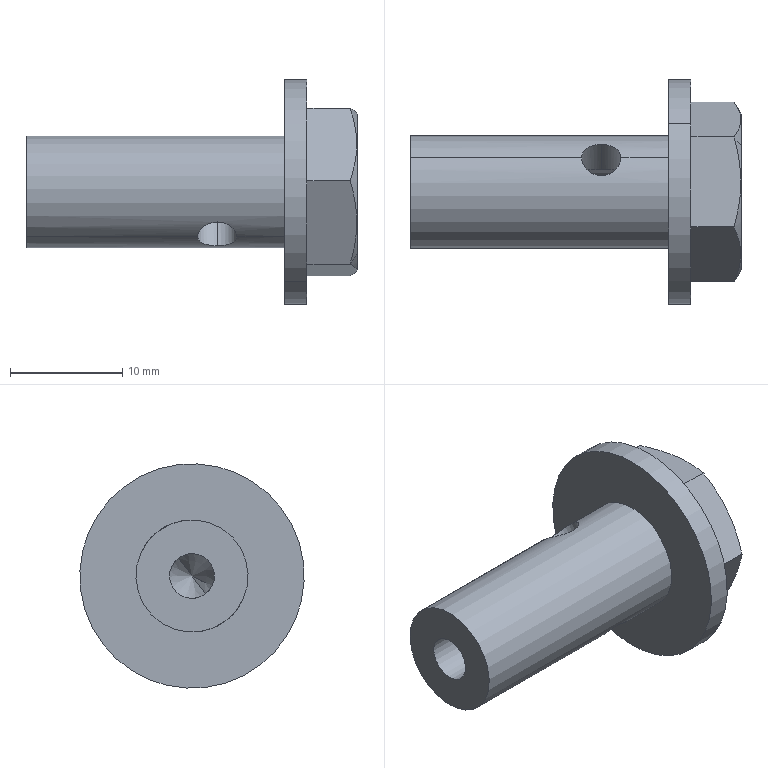Part | SolidWorks | features BaseBody 1 | 1 solid | 24 faces | box 29.5 x 20 x 20 mm | volume 2879 mm3 | cylinder 10 | plane 10 | cone 4 | commonest cylinder face diameters 3.5 x4 4 x2 10 x2 20 x2
STEP:
#1=CARTESIAN_POINT('',(8.537,-14.052,-30.789));
#2=VERTEX_POINT('',#1);
#3=CARTESIAN_POINT('',(8.537,-26.156,-46.711));
#4=VERTEX_POINT('',#3);
#5=CARTESIAN_POINT('',(8.537,-20.104,-38.75));
#6=DIRECTION('',(1.,0.,0.));
#7=DIRECTION('',(0.,0.6052,0.7961));
#8=AXIS2_PLACEMENT_3D('',#5,#6,#7);
#9=CIRCLE('',#8,10.);
#10=EDGE_CURVE('',#2,#4,#9,.T.);
#11=ORIENTED_EDGE('',*,*,#10,.T.);
#12=CARTESIAN_POINT('',(10.537,-26.156,-46.711));
#13=VERTEX_POINT('',#12);
#14=CARTESIAN_POINT('',(15.037,-26.156,-46.711));
#15=DIRECTION('',(1.,0.,0.));
#16=VECTOR('',#15,1000.);
#17=LINE('',#14,#16);
#18=EDGE_CURVE('',#4,#13,#17,.T.);
#19=ORIENTED_EDGE('',*,*,#18,.T.);
#20=CARTESIAN_POINT('',(10.537,-14.052,-30.789));
#21=VERTEX_POINT('',#20);
#22=CARTESIAN_POINT('',(10.537,-20.104,-38.75));
#23=DIRECTION('',(1.,0.,0.));
#24=DIRECTION('',(0.,-0.6052,-0.7961));
#25=AXIS2_PLACEMENT_3D('',#22,#23,#24);
#26=CIRCLE('',#25,10.);
#27=EDGE_CURVE('',#21,#13,#26,.T.);
#28=ORIENTED_EDGE('',*,*,#27,.F.);
#29=CARTESIAN_POINT('',(15.037,-14.052,-30.789));
#30=DIRECTION('',(1.,0.,0.));
#31=VECTOR('',#30,1000.);
#32=LINE('',#29,#31);
#33=EDGE_CURVE('',#2,#21,#32,.T.);
#34=ORIENTED_EDGE('',*,*,#33,.F.);
#35=EDGE_LOOP('',(#11,#19,#28,#34));
#36=FACE_OUTER_BOUND('',#35,.T.);
#37=CARTESIAN_POINT('',(15.037,-20.104,-38.75));
#38=DIRECTION('',(1.,0.,0.));
#39=DIRECTION('',(0.,0.6052,0.7961));
#40=AXIS2_PLACEMENT_3D('',#37,#38,#39);
#41=CYLINDRICAL_SURFACE('',#40,10.);
#42=ADVANCED_FACE('',(#36),#41,.T.);
#43=CARTESIAN_POINT('',(-14.463,-17.078,-34.77));
#44=VERTEX_POINT('',#43);
#45=CARTESIAN_POINT('',(-14.463,-23.13,-42.73));
#46=VERTEX_POINT('',#45);
#47=CARTESIAN_POINT('',(-14.463,-20.104,-38.75));
#48=DIRECTION('',(1.,0.,0.));
#49=DIRECTION('',(0.,0.6052,0.7961));
#50=AXIS2_PLACEMENT_3D('',#47,#48,#49);
#51=CIRCLE('',#50,5.);
#52=EDGE_CURVE('',#44,#46,#51,.T.);
#53=ORIENTED_EDGE('',*,*,#52,.T.);
#54=CARTESIAN_POINT('',(0.7871,-23.13,-42.73));
#55=VERTEX_POINT('',#54);
#56=CARTESIAN_POINT('',(15.037,-23.13,-42.73));
#57=DIRECTION('',(1.,0.,0.));
#58=VECTOR('',#57,1000.);
#59=LINE('',#56,#58);
#60=EDGE_CURVE('',#46,#55,#59,.T.);
#61=ORIENTED_EDGE('',*,*,#60,.T.);
#62=CARTESIAN_POINT('',(2.537,-24.332,-41.419));
#63=VERTEX_POINT('',#62);
#64=CARTESIAN_POINT('',(2.537,-24.332,-41.419));
#65=CARTESIAN_POINT('',(2.42,-24.332,-41.419));
#66=CARTESIAN_POINT('',(2.306,-24.325,-41.43));
#67=CARTESIAN_POINT('',(2.081,-24.299,-41.47));
#68=CARTESIAN_POINT('',(1.97,-24.28,-41.501));
#69=CARTESIAN_POINT('',(1.758,-24.228,-41.578));
#70=CARTESIAN_POINT('',(1.658,-24.195,-41.624));
#71=CARTESIAN_POINT('',(1.469,-24.118,-41.732));
#72=CARTESIAN_POINT('',(1.38,-24.072,-41.793));
#73=CARTESIAN_POINT('',(1.139,-23.918,-41.987));
#74=CARTESIAN_POINT('',(1.01,-23.788,-42.136));
#75=CARTESIAN_POINT('',(0.8778,-23.563,-42.362));
#76=CARTESIAN_POINT('',(0.8437,-23.481,-42.439));
#77=CARTESIAN_POINT('',(0.7984,-23.31,-42.588));
#78=CARTESIAN_POINT('',(0.7871,-23.222,-42.661));
#79=CARTESIAN_POINT('',(0.7871,-23.13,-42.73));
#80=B_SPLINE_CURVE_WITH_KNOTS('',3,(#64,#65,#66,#67,#68,#69,#70,#71,#72,#73,#74,#75,#76,#77,#78,#79),.UNSPECIFIED.,.F.,.F.,(4,2,2,2,2,2,2,4),(0.,0.0003443,0.0006886,0.001033,0.001377,0.002066,0.00241,0.002754),.UNSPECIFIED.);
#81=EDGE_CURVE('',#63,#55,#80,.T.);
#82=ORIENTED_EDGE('',*,*,#81,.F.);
#83=CARTESIAN_POINT('',(4.287,-23.13,-42.73));
#84=VERTEX_POINT('',#83);
#85=CARTESIAN_POINT('',(4.287,-23.13,-42.73));
#86=CARTESIAN_POINT('',(4.287,-23.222,-42.661));
#87=CARTESIAN_POINT('',(4.276,-23.31,-42.588));
#88=CARTESIAN_POINT('',(4.231,-23.481,-42.439));
#89=CARTESIAN_POINT('',(4.197,-23.563,-42.362));
#90=CARTESIAN_POINT('',(4.065,-23.788,-42.137));
#91=CARTESIAN_POINT('',(3.935,-23.918,-41.987));
#92=CARTESIAN_POINT('',(3.695,-24.072,-41.793));
#93=CARTESIAN_POINT('',(3.606,-24.117,-41.732));
#94=CARTESIAN_POINT('',(3.417,-24.195,-41.625));
#95=CARTESIAN_POINT('',(3.316,-24.227,-41.578));
#96=CARTESIAN_POINT('',(3.105,-24.279,-41.501));
#97=CARTESIAN_POINT('',(2.993,-24.299,-41.47));
#98=CARTESIAN_POINT('',(2.768,-24.325,-41.43));
#99=CARTESIAN_POINT('',(2.654,-24.332,-41.419));
#100=CARTESIAN_POINT('',(2.537,-24.332,-41.419));
#101=B_SPLINE_CURVE_WITH_KNOTS('',3,(#85,#86,#87,#88,#89,#90,#91,#92,#93,#94,#95,#96,#97,#98,#99,#100),.UNSPECIFIED.,.F.,.F.,(4,2,2,2,2,2,2,4),(0.008261,0.008606,0.00895,0.009639,0.009983,0.01033,0.01067,0.01102),.UNSPECIFIED.);
#102=EDGE_CURVE('',#84,#63,#101,.T.);
#103=ORIENTED_EDGE('',*,*,#102,.F.);
#104=CARTESIAN_POINT('',(8.537,-23.13,-42.73));
#105=VERTEX_POINT('',#104);
#106=CARTESIAN_POINT('',(15.037,-23.13,-42.73));
#107=DIRECTION('',(1.,0.,0.));
#108=VECTOR('',#107,1000.);
#109=LINE('',#106,#108);
#110=EDGE_CURVE('',#84,#105,#109,.T.);
#111=ORIENTED_EDGE('',*,*,#110,.T.);
#112=CARTESIAN_POINT('',(8.537,-17.078,-34.77));
#113=VERTEX_POINT('',#112);
#114=CARTESIAN_POINT('',(8.537,-20.104,-38.75));
#115=DIRECTION('',(1.,0.,0.));
#116=DIRECTION('',(0.,0.6052,0.7961));
#117=AXIS2_PLACEMENT_3D('',#114,#115,#116);
#118=CIRCLE('',#117,5.);
#119=EDGE_CURVE('',#113,#105,#118,.T.);
#120=ORIENTED_EDGE('',*,*,#119,.F.);
#121=CARTESIAN_POINT('',(4.287,-17.078,-34.77));
#122=VERTEX_POINT('',#121);
#123=CARTESIAN_POINT('',(15.037,-17.078,-34.77));
#124=DIRECTION('',(1.,0.,0.));
#125=VECTOR('',#124,1000.);
#126=LINE('',#123,#125);
#127=EDGE_CURVE('',#122,#113,#126,.T.);
#128=ORIENTED_EDGE('',*,*,#127,.F.);
#129=CARTESIAN_POINT('',(2.537,-18.662,-33.962));
#130=VERTEX_POINT('',#129);
#131=CARTESIAN_POINT('',(2.537,-18.662,-33.962));
#132=CARTESIAN_POINT('',(2.654,-18.662,-33.962));
#133=CARTESIAN_POINT('',(2.768,-18.65,-33.966));
#134=CARTESIAN_POINT('',(2.993,-18.605,-33.98));
#135=CARTESIAN_POINT('',(3.104,-18.57,-33.991));
#136=CARTESIAN_POINT('',(3.316,-18.482,-34.02));
#137=CARTESIAN_POINT('',(3.416,-18.428,-34.039));
#138=CARTESIAN_POINT('',(3.605,-18.305,-34.084));
#139=CARTESIAN_POINT('',(3.694,-18.233,-34.112));
#140=CARTESIAN_POINT('',(3.935,-18.005,-34.209));
#141=CARTESIAN_POINT('',(4.065,-17.826,-34.294));
#142=CARTESIAN_POINT('',(4.196,-17.548,-34.451));
#143=CARTESIAN_POINT('',(4.231,-17.453,-34.509));
#144=CARTESIAN_POINT('',(4.276,-17.263,-34.634));
#145=CARTESIAN_POINT('',(4.287,-17.17,-34.7));
#146=CARTESIAN_POINT('',(4.287,-17.078,-34.77));
#147=B_SPLINE_CURVE_WITH_KNOTS('',3,(#131,#132,#133,#134,#135,#136,#137,#138,#139,#140,#141,#142,#143,#144,#145,#146),.UNSPECIFIED.,.F.,.F.,(4,2,2,2,2,2,2,4),(0.,0.0003443,0.0006886,0.001033,0.001377,0.002066,0.00241,0.002754),.UNSPECIFIED.);
#148=EDGE_CURVE('',#130,#122,#147,.T.);
#149=ORIENTED_EDGE('',*,*,#148,.F.);
#150=CARTESIAN_POINT('',(0.7871,-17.078,-34.77));
#151=VERTEX_POINT('',#150);
#152=CARTESIAN_POINT('',(0.7871,-17.078,-34.77));
#153=CARTESIAN_POINT('',(0.7871,-17.17,-34.7));
#154=CARTESIAN_POINT('',(0.7984,-17.263,-34.634));
#155=CARTESIAN_POINT('',(0.8436,-17.453,-34.509));
#156=CARTESIAN_POINT('',(0.8777,-17.548,-34.451));
#157=CARTESIAN_POINT('',(1.009,-17.825,-34.294));
#158=CARTESIAN_POINT('',(1.139,-18.004,-34.209));
#159=CARTESIAN_POINT('',(1.379,-18.233,-34.113));
#160=CARTESIAN_POINT('',(1.468,-18.304,-34.085));
#161=CARTESIAN_POINT('',(1.658,-18.428,-34.039));
#162=CARTESIAN_POINT('',(1.758,-18.482,-34.02));
#163=CARTESIAN_POINT('',(1.969,-18.57,-33.991));
#164=CARTESIAN_POINT('',(2.081,-18.605,-33.98));
#165=CARTESIAN_POINT('',(2.306,-18.65,-33.966));
#166=CARTESIAN_POINT('',(2.42,-18.662,-33.962));
#167=CARTESIAN_POINT('',(2.537,-18.662,-33.962));
#168=B_SPLINE_CURVE_WITH_KNOTS('',3,(#152,#153,#154,#155,#156,#157,#158,#159,#160,#161,#162,#163,#164,#165,#166,#167),.UNSPECIFIED.,.F.,.F.,(4,2,2,2,2,2,2,4),(0.008261,0.008606,0.00895,0.009639,0.009983,0.01033,0.01067,0.01102),.UNSPECIFIED.);
#169=EDGE_CURVE('',#151,#130,#168,.T.);
#170=ORIENTED_EDGE('',*,*,#169,.F.);
#171=CARTESIAN_POINT('',(15.037,-17.078,-34.77));
#172=DIRECTION('',(1.,0.,0.));
#173=VECTOR('',#172,1000.);
#174=LINE('',#171,#173);
#175=EDGE_CURVE('',#44,#151,#174,.T.);
#176=ORIENTED_EDGE('',*,*,#175,.F.);
#177=EDGE_LOOP('',(#53,#61,#82,#103,#111,#120,#128,#149,#170,#176));
#178=FACE_OUTER_BOUND('',#177,.T.);
#179=CARTESIAN_POINT('',(15.037,-20.104,-38.75));
#180=DIRECTION('',(1.,0.,0.));
#181=DIRECTION('',(0.,0.6052,0.7961));
#182=AXIS2_PLACEMENT_3D('',#179,#180,#181);
#183=CYLINDRICAL_SURFACE('',#182,5.);
#184=ADVANCED_FACE('',(#178),#183,.T.);
#185=CARTESIAN_POINT('',(-14.463,-21.314,-40.342));
#186=VERTEX_POINT('',#185);
#187=CARTESIAN_POINT('',(-14.463,-18.893,-37.158));
#188=VERTEX_POINT('',#187);
#189=CARTESIAN_POINT('',(-14.463,-20.104,-38.75));
#190=DIRECTION('',(1.,0.,0.));
#191=DIRECTION('',(0.,0.6052,0.7961));
#192=AXIS2_PLACEMENT_3D('',#189,#190,#191);
#193=CIRCLE('',#192,2.);
#194=EDGE_CURVE('',#186,#188,#193,.T.);
#195=ORIENTED_EDGE('',*,*,#194,.F.);
#196=CARTESIAN_POINT('',(0.7871,-21.314,-40.342));
#197=VERTEX_POINT('',#196);
#198=CARTESIAN_POINT('',(15.037,-21.314,-40.342));
#199=DIRECTION('',(1.,0.,0.));
#200=VECTOR('',#199,1000.);
#201=LINE('',#198,#200);
#202=EDGE_CURVE('',#186,#197,#201,.T.);
#203=ORIENTED_EDGE('',*,*,#202,.T.);
#204=CARTESIAN_POINT('',(2.537,-19.297,-40.58));
#205=VERTEX_POINT('',#204);
#206=CARTESIAN_POINT('',(2.537,-19.297,-40.58));
#207=CARTESIAN_POINT('',(2.414,-19.297,-40.58));
#208=CARTESIAN_POINT('',(2.289,-19.323,-40.592));
#209=CARTESIAN_POINT('',(2.06,-19.41,-40.626));
#210=CARTESIAN_POINT('',(1.952,-19.471,-40.649));
#211=CARTESIAN_POINT('',(1.65,-19.679,-40.71));
#212=CARTESIAN_POINT('',(1.472,-19.854,-40.744));
#213=CARTESIAN_POINT('',(1.241,-20.143,-40.752));
#214=CARTESIAN_POINT('',(1.17,-20.243,-40.748));
#215=CARTESIAN_POINT('',(1.041,-20.454,-40.722));
#216=CARTESIAN_POINT('',(0.9837,-20.563,-40.7));
#217=CARTESIAN_POINT('',(0.8893,-20.782,-40.635));
#218=CARTESIAN_POINT('',(0.8512,-20.895,-40.591));
#219=CARTESIAN_POINT('',(0.8004,-21.111,-40.482));
#220=CARTESIAN_POINT('',(0.7871,-21.215,-40.418));
#221=CARTESIAN_POINT('',(0.7871,-21.314,-40.342));
#222=B_SPLINE_CURVE_WITH_KNOTS('',3,(#206,#207,#208,#209,#210,#211,#212,#213,#214,#215,#216,#217,#218,#219,#220,#221),.UNSPECIFIED.,.F.,.F.,(4,2,2,2,2,2,2,4),(0.005929,0.006299,0.00667,0.007412,0.007783,0.008154,0.008525,0.008895),.UNSPECIFIED.);
#223=EDGE_CURVE('',#205,#197,#222,.T.);
#224=ORIENTED_EDGE('',*,*,#223,.F.);
#225=CARTESIAN_POINT('',(4.287,-21.314,-40.342));
#226=VERTEX_POINT('',#225);
#227=CARTESIAN_POINT('',(4.287,-21.314,-40.342));
#228=CARTESIAN_POINT('',(4.287,-21.216,-40.417));
#229=CARTESIAN_POINT('',(4.274,-21.109,-40.483));
#230=CARTESIAN_POINT('',(4.223,-20.893,-40.592));
#231=CARTESIAN_POINT('',(4.185,-20.782,-40.635));
#232=CARTESIAN_POINT('',(4.042,-20.452,-40.733));
#233=CARTESIAN_POINT('',(3.909,-20.237,-40.755));
#234=CARTESIAN_POINT('',(3.601,-19.853,-40.744));
#235=CARTESIAN_POINT('',(3.423,-19.678,-40.709));
#236=CARTESIAN_POINT('',(3.122,-19.471,-40.649));
#237=CARTESIAN_POINT('',(3.014,-19.41,-40.627));
#238=CARTESIAN_POINT('',(2.785,-19.323,-40.592));
#239=CARTESIAN_POINT('',(2.66,-19.297,-40.58));
#240=CARTESIAN_POINT('',(2.537,-19.297,-40.58));
#241=B_SPLINE_CURVE_WITH_KNOTS('',3,(#227,#228,#229,#230,#231,#232,#233,#234,#235,#236,#237,#238,#239,#240),.UNSPECIFIED.,.F.,.F.,(4,2,2,2,2,2,4),(0.002967,0.003337,0.003707,0.004448,0.005188,0.005558,0.005929),.UNSPECIFIED.);
#242=EDGE_CURVE('',#226,#205,#241,.T.);
#243=ORIENTED_EDGE('',*,*,#242,.F.);
#244=CARTESIAN_POINT('',(4.537,-21.314,-40.342));
#245=VERTEX_POINT('',#244);
#246=CARTESIAN_POINT('',(15.037,-21.314,-40.342));
#247=DIRECTION('',(1.,0.,0.));
#248=VECTOR('',#247,1000.);
#249=LINE('',#246,#248);
#250=EDGE_CURVE('',#226,#245,#249,.T.);
#251=ORIENTED_EDGE('',*,*,#250,.T.);
#252=CARTESIAN_POINT('',(4.537,-18.893,-37.158));
#253=VERTEX_POINT('',#252);
#254=CARTESIAN_POINT('',(4.537,-20.104,-38.75));
#255=DIRECTION('',(1.,0.,0.));
#256=DIRECTION('',(0.,0.6052,0.7961));
#257=AXIS2_PLACEMENT_3D('',#254,#255,#256);
#258=CIRCLE('',#257,2.);
#259=EDGE_CURVE('',#245,#253,#258,.T.);
#260=ORIENTED_EDGE('',*,*,#259,.T.);
#261=CARTESIAN_POINT('',(4.287,-18.893,-37.158));
#262=VERTEX_POINT('',#261);
#263=CARTESIAN_POINT('',(15.037,-18.893,-37.158));
#264=DIRECTION('',(1.,0.,0.));
#265=VECTOR('',#264,1000.);
#266=LINE('',#263,#265);
#267=EDGE_CURVE('',#262,#253,#266,.T.);
#268=ORIENTED_EDGE('',*,*,#267,.F.);
#269=CARTESIAN_POINT('',(2.537,-18.125,-39.038));
#270=VERTEX_POINT('',#269);
#271=CARTESIAN_POINT('',(2.537,-18.125,-39.038));
#272=CARTESIAN_POINT('',(2.661,-18.125,-39.038));
#273=CARTESIAN_POINT('',(2.785,-18.12,-39.01));
#274=CARTESIAN_POINT('',(3.014,-18.11,-38.916));
#275=CARTESIAN_POINT('',(3.123,-18.105,-38.852));
#276=CARTESIAN_POINT('',(3.424,-18.102,-38.635));
#277=CARTESIAN_POINT('',(3.602,-18.116,-38.457));
#278=CARTESIAN_POINT('',(3.833,-18.185,-38.177));
#279=CARTESIAN_POINT('',(3.904,-18.216,-38.081));
#280=CARTESIAN_POINT('',(4.033,-18.297,-37.885));
#281=CARTESIAN_POINT('',(4.091,-18.348,-37.786));
#282=CARTESIAN_POINT('',(4.185,-18.469,-37.592));
#283=CARTESIAN_POINT('',(4.223,-18.541,-37.496));
#284=CARTESIAN_POINT('',(4.274,-18.704,-37.317));
#285=CARTESIAN_POINT('',(4.287,-18.794,-37.234));
#286=CARTESIAN_POINT('',(4.287,-18.893,-37.158));
#287=B_SPLINE_CURVE_WITH_KNOTS('',3,(#271,#272,#273,#274,#275,#276,#277,#278,#279,#280,#281,#282,#283,#284,#285,#286),.UNSPECIFIED.,.F.,.F.,(4,2,2,2,2,2,2,4),(0.005929,0.006299,0.00667,0.007412,0.007783,0.008154,0.008525,0.008895),.UNSPECIFIED.);
#288=EDGE_CURVE('',#270,#262,#287,.T.);
#289=ORIENTED_EDGE('',*,*,#288,.F.);
#290=CARTESIAN_POINT('',(0.7871,-18.893,-37.158));
#291=VERTEX_POINT('',#290);
#292=CARTESIAN_POINT('',(0.7871,-18.893,-37.158));
#293=CARTESIAN_POINT('',(0.7871,-18.795,-37.232));
#294=CARTESIAN_POINT('',(0.8006,-18.703,-37.318));
#295=CARTESIAN_POINT('',(0.8516,-18.54,-37.497));
#296=CARTESIAN_POINT('',(0.8894,-18.469,-37.593));
#297=CARTESIAN_POINT('',(1.032,-18.286,-37.885));
#298=CARTESIAN_POINT('',(1.165,-18.208,-38.085));
#299=CARTESIAN_POINT('',(1.473,-18.116,-38.458));
#300=CARTESIAN_POINT('',(1.651,-18.102,-38.636));
#301=CARTESIAN_POINT('',(1.952,-18.105,-38.852));
#302=CARTESIAN_POINT('',(2.06,-18.11,-38.916));
#303=CARTESIAN_POINT('',(2.29,-18.12,-39.01));
#304=CARTESIAN_POINT('',(2.414,-18.125,-39.038));
#305=CARTESIAN_POINT('',(2.537,-18.125,-39.038));
#306=B_SPLINE_CURVE_WITH_KNOTS('',3,(#292,#293,#294,#295,#296,#297,#298,#299,#300,#301,#302,#303,#304,#305),.UNSPECIFIED.,.F.,.F.,(4,2,2,2,2,2,4),(0.002967,0.003337,0.003707,0.004448,0.005188,0.005558,0.005929),.UNSPECIFIED.);
#307=EDGE_CURVE('',#291,#270,#306,.T.);
#308=ORIENTED_EDGE('',*,*,#307,.F.);
#309=CARTESIAN_POINT('',(15.037,-18.893,-37.158));
#310=DIRECTION('',(1.,0.,0.));
#311=VECTOR('',#310,1000.);
#312=LINE('',#309,#311);
#313=EDGE_CURVE('',#188,#291,#312,.T.);
#314=ORIENTED_EDGE('',*,*,#313,.F.);
#315=EDGE_LOOP('',(#195,#203,#224,#243,#251,#260,#268,#289,#308,#314));
#316=FACE_OUTER_BOUND('',#315,.T.);
#317=CARTESIAN_POINT('',(15.037,-20.104,-38.75));
#318=DIRECTION('',(1.,0.,0.));
#319=DIRECTION('',(0.,0.6052,0.7961));
#320=AXIS2_PLACEMENT_3D('',#317,#318,#319);
#321=CYLINDRICAL_SURFACE('',#320,2.);
#322=ADVANCED_FACE('',(#316),#321,.F.);
#323=CARTESIAN_POINT('',(8.537,-20.104,-38.75));
#324=VERTEX_POINT('',#323);
#325=CARTESIAN_POINT('',(4.537,-21.314,-40.342));
#326=DIRECTION('',(-0.8944,-0.2707,-0.356));
#327=VECTOR('',#326,1000.);
#328=LINE('',#325,#327);
#329=EDGE_CURVE('',#324,#245,#328,.T.);
#330=ORIENTED_EDGE('',*,*,#329,.F.);
#331=CARTESIAN_POINT('',(4.537,-18.893,-37.158));
#332=DIRECTION('',(-0.8944,0.2707,0.356));
#333=VECTOR('',#332,1000.);
#334=LINE('',#331,#333);
#335=EDGE_CURVE('',#324,#253,#334,.T.);
#336=ORIENTED_EDGE('',*,*,#335,.T.);
#337=ORIENTED_EDGE('',*,*,#259,.F.);
#338=EDGE_LOOP('',(#330,#336,#337));
#339=FACE_OUTER_BOUND('',#338,.T.);
#340=CARTESIAN_POINT('',(4.537,-20.104,-38.75));
#341=DIRECTION('',(-1.,0.,0.));
#342=DIRECTION('',(0.,-0.6052,-0.7961));
#343=AXIS2_PLACEMENT_3D('',#340,#341,#342);
#344=CONICAL_SURFACE('',#343,2.,0.4636);
#345=ADVANCED_FACE('',(#339),#344,.F.);
#346=CARTESIAN_POINT('',(15.037,-24.275,-44.236));
#347=VERTEX_POINT('',#346);
#348=CARTESIAN_POINT('',(15.037,-15.933,-33.264));
#349=VERTEX_POINT('',#348);
#350=CARTESIAN_POINT('',(15.037,-20.104,-38.75));
#351=DIRECTION('',(1.,0.,0.));
#352=DIRECTION('',(0.,0.6052,0.7961));
#353=AXIS2_PLACEMENT_3D('',#350,#351,#352);
#354=CIRCLE('',#353,6.892);
#355=EDGE_CURVE('',#347,#349,#354,.T.);
#356=ORIENTED_EDGE('',*,*,#355,.F.);
#357=CARTESIAN_POINT('',(14.377,-24.996,-45.185));
#358=VERTEX_POINT('',#357);
#359=CARTESIAN_POINT('',(15.037,-24.275,-44.236));
#360=DIRECTION('',(-0.4848,-0.5293,-0.6963));
#361=VECTOR('',#360,1000.);
#362=LINE('',#359,#361);
#363=EDGE_CURVE('',#347,#358,#362,.T.);
#364=ORIENTED_EDGE('',*,*,#363,.T.);
#365=CARTESIAN_POINT('',(14.377,-16.977,-46.204));
#366=VERTEX_POINT('',#365);
#367=CARTESIAN_POINT('',(14.377,-16.977,-46.204));
#368=CARTESIAN_POINT('',(14.56,-17.633,-46.12));
#369=CARTESIAN_POINT('',(14.711,-18.293,-46.036));
#370=CARTESIAN_POINT('',(14.919,-19.626,-45.867));
#371=CARTESIAN_POINT('',(14.977,-20.299,-45.782));
#372=CARTESIAN_POINT('',(14.977,-21.32,-45.652));
#373=CARTESIAN_POINT('',(14.963,-21.662,-45.608));
#374=CARTESIAN_POINT('',(14.909,-22.339,-45.522));
#375=CARTESIAN_POINT('',(14.868,-22.675,-45.48));
#376=CARTESIAN_POINT('',(14.711,-23.678,-45.352));
#377=CARTESIAN_POINT('',(14.56,-24.339,-45.268));
#378=CARTESIAN_POINT('',(14.377,-24.996,-45.185));
#379=B_SPLINE_CURVE_WITH_KNOTS('',3,(#367,#368,#369,#370,#371,#372,#373,#374,#375,#376,#377,#378),.UNSPECIFIED.,.F.,.F.,(4,2,2,2,2,4),(0.,0.00204,0.004079,0.005099,0.006119,0.008158),.UNSPECIFIED.);
#380=EDGE_CURVE('',#366,#358,#379,.T.);
#381=ORIENTED_EDGE('',*,*,#380,.F.);
#382=CARTESIAN_POINT('',(14.377,-12.085,-39.769));
#383=VERTEX_POINT('',#382);
#384=CARTESIAN_POINT('',(14.377,-12.085,-39.769));
#385=CARTESIAN_POINT('',(14.56,-12.485,-40.295));
#386=CARTESIAN_POINT('',(14.711,-12.888,-40.825));
#387=CARTESIAN_POINT('',(14.919,-13.701,-41.895));
#388=CARTESIAN_POINT('',(14.977,-14.112,-42.435));
#389=CARTESIAN_POINT('',(14.977,-14.735,-43.254));
#390=CARTESIAN_POINT('',(14.963,-14.943,-43.529));
#391=CARTESIAN_POINT('',(14.909,-15.356,-44.071));
#392=CARTESIAN_POINT('',(14.868,-15.561,-44.341));
#393=CARTESIAN_POINT('',(14.711,-16.173,-45.146));
#394=CARTESIAN_POINT('',(14.56,-16.577,-45.677));
#395=CARTESIAN_POINT('',(14.377,-16.977,-46.204));
#396=B_SPLINE_CURVE_WITH_KNOTS('',3,(#384,#385,#386,#387,#388,#389,#390,#391,#392,#393,#394,#395),.UNSPECIFIED.,.F.,.F.,(4,2,2,2,2,4),(0.,0.00204,0.004079,0.005099,0.006119,0.008158),.UNSPECIFIED.);
#397=EDGE_CURVE('',#383,#366,#396,.T.);
#398=ORIENTED_EDGE('',*,*,#397,.F.);
#399=CARTESIAN_POINT('',(14.377,-15.212,-32.315));
#400=VERTEX_POINT('',#399);
#401=CARTESIAN_POINT('',(14.377,-15.212,-32.315));
#402=CARTESIAN_POINT('',(14.56,-14.956,-32.925));
#403=CARTESIAN_POINT('',(14.711,-14.699,-33.539));
#404=CARTESIAN_POINT('',(14.919,-14.179,-34.778));
#405=CARTESIAN_POINT('',(14.977,-13.917,-35.403));
#406=CARTESIAN_POINT('',(14.977,-13.519,-36.353));
#407=CARTESIAN_POINT('',(14.963,-13.385,-36.67));
#408=CARTESIAN_POINT('',(14.909,-13.121,-37.299));
#409=CARTESIAN_POINT('',(14.868,-12.99,-37.612));
#410=CARTESIAN_POINT('',(14.711,-12.599,-38.544));
#411=CARTESIAN_POINT('',(14.56,-12.341,-39.159));
#412=CARTESIAN_POINT('',(14.377,-12.085,-39.769));
#413=B_SPLINE_CURVE_WITH_KNOTS('',3,(#401,#402,#403,#404,#405,#406,#407,#408,#409,#410,#411,#412),.UNSPECIFIED.,.F.,.F.,(4,2,2,2,2,4),(0.,0.00204,0.004079,0.005099,0.006119,0.008158),.UNSPECIFIED.);
#414=EDGE_CURVE('',#400,#383,#413,.T.);
#415=ORIENTED_EDGE('',*,*,#414,.F.);
#416=CARTESIAN_POINT('',(15.037,-15.933,-33.264));
#417=DIRECTION('',(-0.4848,0.5293,0.6963));
#418=VECTOR('',#417,1000.);
#419=LINE('',#416,#418);
#420=EDGE_CURVE('',#349,#400,#419,.T.);
#421=ORIENTED_EDGE('',*,*,#420,.F.);
#422=EDGE_LOOP('',(#356,#364,#381,#398,#415,#421));
#423=FACE_OUTER_BOUND('',#422,.T.);
#424=CARTESIAN_POINT('',(15.037,-20.104,-38.75));
#425=DIRECTION('',(-1.,0.,0.));
#426=DIRECTION('',(0.,0.6052,0.7961));
#427=AXIS2_PLACEMENT_3D('',#424,#425,#426);
#428=CONICAL_SURFACE('',#427,6.892,1.065);
#429=ADVANCED_FACE('',(#423),#428,.T.);
#430=CARTESIAN_POINT('',(2.537,-22.083,-38.462));
#431=VERTEX_POINT('',#430);
#432=CARTESIAN_POINT('',(2.537,-22.083,-38.462));
#433=CARTESIAN_POINT('',(2.663,-22.083,-38.462));
#434=CARTESIAN_POINT('',(2.784,-22.087,-38.49));
#435=CARTESIAN_POINT('',(3.015,-22.097,-38.584));
#436=CARTESIAN_POINT('',(3.122,-22.102,-38.647));
#437=CARTESIAN_POINT('',(3.323,-22.105,-38.792));
#438=CARTESIAN_POINT('',(3.418,-22.102,-38.874));
#439=CARTESIAN_POINT('',(3.595,-22.084,-39.044));
#440=CARTESIAN_POINT('',(3.677,-22.069,-39.134));
#441=CARTESIAN_POINT('',(3.91,-22.,-39.416));
#442=CARTESIAN_POINT('',(4.042,-21.922,-39.615));
#443=CARTESIAN_POINT('',(4.185,-21.738,-39.908));
#444=CARTESIAN_POINT('',(4.222,-21.668,-40.003));
#445=CARTESIAN_POINT('',(4.274,-21.504,-40.183));
#446=CARTESIAN_POINT('',(4.287,-21.412,-40.268));
#447=CARTESIAN_POINT('',(4.287,-21.314,-40.342));
#448=B_SPLINE_CURVE_WITH_KNOTS('',3,(#432,#433,#434,#435,#436,#437,#438,#439,#440,#441,#442,#443,#444,#445,#446,#447),.UNSPECIFIED.,.F.,.F.,(4,2,2,2,2,2,2,4),(0.,0.0003708,0.0007416,0.001112,0.001483,0.002225,0.002596,0.002967),.UNSPECIFIED.);
#449=EDGE_CURVE('',#431,#226,#448,.T.);
#450=ORIENTED_EDGE('',*,*,#449,.T.);
#451=ORIENTED_EDGE('',*,*,#242,.T.);
#452=CARTESIAN_POINT('',(2.537,-21.545,-43.538));
#453=VERTEX_POINT('',#452);
#454=CARTESIAN_POINT('',(2.537,-12.659,-31.848));
#455=DIRECTION('',(0.,-0.6052,-0.7961));
#456=VECTOR('',#455,1000.);
#457=LINE('',#454,#456);
#458=EDGE_CURVE('',#205,#453,#457,.T.);
#459=ORIENTED_EDGE('',*,*,#458,.T.);
#460=CARTESIAN_POINT('',(2.537,-21.545,-43.538));
#461=CARTESIAN_POINT('',(2.767,-21.545,-43.538));
#462=CARTESIAN_POINT('',(2.999,-21.593,-43.524));
#463=CARTESIAN_POINT('',(3.314,-21.725,-43.48));
#464=CARTESIAN_POINT('',(3.416,-21.78,-43.461));
#465=CARTESIAN_POINT('',(3.605,-21.904,-43.415));
#466=CARTESIAN_POINT('',(3.693,-21.973,-43.388));
#467=CARTESIAN_POINT('',(3.854,-22.126,-43.324));
#468=CARTESIAN_POINT('',(3.927,-22.209,-43.286));
#469=CARTESIAN_POINT('',(4.054,-22.382,-43.202));
#470=CARTESIAN_POINT('',(4.108,-22.473,-43.155));
#471=CARTESIAN_POINT('',(4.197,-22.66,-43.049));
#472=CARTESIAN_POINT('',(4.23,-22.754,-42.991));
#473=CARTESIAN_POINT('',(4.275,-22.943,-42.868));
#474=CARTESIAN_POINT('',(4.287,-23.038,-42.8));
#475=CARTESIAN_POINT('',(4.287,-23.13,-42.73));
#476=B_SPLINE_CURVE_WITH_KNOTS('',3,(#460,#461,#462,#463,#464,#465,#466,#467,#468,#469,#470,#471,#472,#473,#474,#475),.UNSPECIFIED.,.F.,.F.,(4,2,2,2,2,2,2,4),(0.005508,0.006196,0.00654,0.006884,0.007229,0.007573,0.007917,0.008261),.UNSPECIFIED.);
#477=EDGE_CURVE('',#453,#84,#476,.T.);
#478=ORIENTED_EDGE('',*,*,#477,.T.);
#479=ORIENTED_EDGE('',*,*,#102,.T.);
#480=CARTESIAN_POINT('',(2.537,-15.445,-29.73));
#481=DIRECTION('',(0.,-0.6052,-0.7961));
#482=VECTOR('',#481,1000.);
#483=LINE('',#480,#482);
#484=EDGE_CURVE('',#431,#63,#483,.T.);
#485=ORIENTED_EDGE('',*,*,#484,.F.);
#486=EDGE_LOOP('',(#450,#451,#459,#478,#479,#485));
#487=FACE_OUTER_BOUND('',#486,.T.);
#488=CARTESIAN_POINT('',(2.537,-14.052,-30.789));
#489=DIRECTION('',(0.,-0.6052,-0.7961));
#490=DIRECTION('',(0.,-0.7961,0.6052));
#491=AXIS2_PLACEMENT_3D('',#488,#489,#490);
#492=CYLINDRICAL_SURFACE('',#491,1.75);
#493=ADVANCED_FACE('',(#487),#492,.F.);
#494=ORIENTED_EDGE('',*,*,#148,.T.);
#495=CARTESIAN_POINT('',(2.537,-15.876,-36.081));
#496=VERTEX_POINT('',#495);
#497=CARTESIAN_POINT('',(4.287,-17.078,-34.77));
#498=CARTESIAN_POINT('',(4.287,-16.986,-34.839));
#499=CARTESIAN_POINT('',(4.275,-16.895,-34.913));
#500=CARTESIAN_POINT('',(4.23,-16.726,-35.062));
#501=CARTESIAN_POINT('',(4.197,-16.646,-35.137));
#502=CARTESIAN_POINT('',(4.064,-16.418,-35.364));
#503=CARTESIAN_POINT('',(3.936,-16.29,-35.512));
#504=CARTESIAN_POINT('',(3.694,-16.135,-35.708));
#505=CARTESIAN_POINT('',(3.606,-16.09,-35.768));
#506=CARTESIAN_POINT('',(3.417,-16.013,-35.875));
#507=CARTESIAN_POINT('',(3.315,-15.98,-35.922));
#508=CARTESIAN_POINT('',(2.998,-15.902,-36.038));
#509=CARTESIAN_POINT('',(2.767,-15.876,-36.081));
#510=CARTESIAN_POINT('',(2.537,-15.876,-36.081));
#511=B_SPLINE_CURVE_WITH_KNOTS('',3,(#497,#498,#499,#500,#501,#502,#503,#504,#505,#506,#507,#508,#509,#510),.UNSPECIFIED.,.F.,.F.,(4,2,2,2,2,2,4),(0.002754,0.003098,0.003443,0.004131,0.004475,0.004819,0.005508),.UNSPECIFIED.);
#512=EDGE_CURVE('',#122,#496,#511,.T.);
#513=ORIENTED_EDGE('',*,*,#512,.T.);
#514=CARTESIAN_POINT('',(2.537,-12.659,-31.848));
#515=DIRECTION('',(0.,-0.6052,-0.7961));
#516=VECTOR('',#515,1000.);
#517=LINE('',#514,#516);
#518=EDGE_CURVE('',#496,#270,#517,.T.);
#519=ORIENTED_EDGE('',*,*,#518,.T.);
#520=ORIENTED_EDGE('',*,*,#288,.T.);
#521=CARTESIAN_POINT('',(2.537,-20.911,-36.92));
#522=VERTEX_POINT('',#521);
#523=CARTESIAN_POINT('',(4.287,-18.893,-37.158));
#524=CARTESIAN_POINT('',(4.287,-18.993,-37.082));
#525=CARTESIAN_POINT('',(4.274,-19.098,-37.017));
#526=CARTESIAN_POINT('',(4.223,-19.314,-36.908));
#527=CARTESIAN_POINT('',(4.185,-19.426,-36.865));
#528=CARTESIAN_POINT('',(4.09,-19.645,-36.8));
#529=CARTESIAN_POINT('',(4.032,-19.755,-36.778));
#530=CARTESIAN_POINT('',(3.904,-19.964,-36.752));
#531=CARTESIAN_POINT('',(3.833,-20.065,-36.748));
#532=CARTESIAN_POINT('',(3.678,-20.258,-36.754));
#533=CARTESIAN_POINT('',(3.595,-20.35,-36.763));
#534=CARTESIAN_POINT('',(3.418,-20.52,-36.792));
#535=CARTESIAN_POINT('',(3.324,-20.598,-36.811));
#536=CARTESIAN_POINT('',(3.122,-20.737,-36.851));
#537=CARTESIAN_POINT('',(3.015,-20.797,-36.873));
#538=CARTESIAN_POINT('',(2.785,-20.885,-36.908));
#539=CARTESIAN_POINT('',(2.663,-20.911,-36.92));
#540=CARTESIAN_POINT('',(2.537,-20.911,-36.92));
#541=B_SPLINE_CURVE_WITH_KNOTS('',3,(#523,#524,#525,#526,#527,#528,#529,#530,#531,#532,#533,#534,#535,#536,#537,#538,#539,#540),.UNSPECIFIED.,.F.,.F.,(4,2,2,2,2,2,2,2,4),(0.008895,0.009266,0.009636,0.01001,0.01038,0.01075,0.01112,0.01149,0.01186),.UNSPECIFIED.);
#542=EDGE_CURVE('',#262,#522,#541,.T.);
#543=ORIENTED_EDGE('',*,*,#542,.T.);
#544=CARTESIAN_POINT('',(2.537,-15.445,-29.73));
#545=DIRECTION('',(0.,-0.6052,-0.7961));
#546=VECTOR('',#545,1000.);
#547=LINE('',#544,#546);
#548=EDGE_CURVE('',#130,#522,#547,.T.);
#549=ORIENTED_EDGE('',*,*,#548,.F.);
#550=EDGE_LOOP('',(#494,#513,#519,#520,#543,#549));
#551=FACE_OUTER_BOUND('',#550,.T.);
#552=CARTESIAN_POINT('',(2.537,-14.052,-30.789));
#553=DIRECTION('',(0.,-0.6052,-0.7961));
#554=DIRECTION('',(0.,-0.7961,0.6052));
#555=AXIS2_PLACEMENT_3D('',#552,#553,#554);
#556=CYLINDRICAL_SURFACE('',#555,1.75);
#557=ADVANCED_FACE('',(#551),#556,.F.);
#558=ORIENTED_EDGE('',*,*,#518,.F.);
#559=CARTESIAN_POINT('',(2.537,-15.876,-36.081));
#560=CARTESIAN_POINT('',(2.307,-15.876,-36.081));
#561=CARTESIAN_POINT('',(2.076,-15.902,-36.038));
#562=CARTESIAN_POINT('',(1.76,-15.98,-35.923));
#563=CARTESIAN_POINT('',(1.658,-16.012,-35.875));
#564=CARTESIAN_POINT('',(1.469,-16.09,-35.768));
#565=CARTESIAN_POINT('',(1.381,-16.135,-35.708));
#566=CARTESIAN_POINT('',(1.22,-16.238,-35.578));
#567=CARTESIAN_POINT('',(1.147,-16.296,-35.508));
#568=CARTESIAN_POINT('',(1.021,-16.423,-35.364));
#569=CARTESIAN_POINT('',(0.9663,-16.493,-35.29));
#570=CARTESIAN_POINT('',(0.8775,-16.645,-35.137));
#571=CARTESIAN_POINT('',(0.844,-16.726,-35.062));
#572=CARTESIAN_POINT('',(0.7988,-16.895,-34.913));
#573=CARTESIAN_POINT('',(0.7871,-16.986,-34.839));
#574=CARTESIAN_POINT('',(0.7871,-17.078,-34.77));
#575=B_SPLINE_CURVE_WITH_KNOTS('',3,(#559,#560,#561,#562,#563,#564,#565,#566,#567,#568,#569,#570,#571,#572,#573,#574),.UNSPECIFIED.,.F.,.F.,(4,2,2,2,2,2,2,4),(0.005508,0.006196,0.00654,0.006884,0.007229,0.007573,0.007917,0.008261),.UNSPECIFIED.);
#576=EDGE_CURVE('',#496,#151,#575,.T.);
#577=ORIENTED_EDGE('',*,*,#576,.T.);
#578=ORIENTED_EDGE('',*,*,#169,.T.);
#579=ORIENTED_EDGE('',*,*,#548,.T.);
#580=CARTESIAN_POINT('',(2.537,-20.911,-36.92));
#581=CARTESIAN_POINT('',(2.411,-20.911,-36.92));
#582=CARTESIAN_POINT('',(2.29,-20.885,-36.908));
#583=CARTESIAN_POINT('',(2.059,-20.797,-36.873));
#584=CARTESIAN_POINT('',(1.953,-20.737,-36.852));
#585=CARTESIAN_POINT('',(1.751,-20.598,-36.811));
#586=CARTESIAN_POINT('',(1.656,-20.519,-36.792));
#587=CARTESIAN_POINT('',(1.479,-20.35,-36.763));
#588=CARTESIAN_POINT('',(1.397,-20.259,-36.754));
#589=CARTESIAN_POINT('',(1.164,-19.97,-36.745));
#590=CARTESIAN_POINT('',(1.032,-19.757,-36.767));
#591=CARTESIAN_POINT('',(0.889,-19.425,-36.865));
#592=CARTESIAN_POINT('',(0.8518,-19.315,-36.908));
#593=CARTESIAN_POINT('',(0.8005,-19.098,-37.017));
#594=CARTESIAN_POINT('',(0.7871,-18.992,-37.083));
#595=CARTESIAN_POINT('',(0.7871,-18.893,-37.158));
#596=B_SPLINE_CURVE_WITH_KNOTS('',3,(#580,#581,#582,#583,#584,#585,#586,#587,#588,#589,#590,#591,#592,#593,#594,#595),.UNSPECIFIED.,.F.,.F.,(4,2,2,2,2,2,2,4),(0.,0.0003708,0.0007416,0.001112,0.001483,0.002225,0.002596,0.002967),.UNSPECIFIED.);
#597=EDGE_CURVE('',#522,#291,#596,.T.);
#598=ORIENTED_EDGE('',*,*,#597,.T.);
#599=ORIENTED_EDGE('',*,*,#307,.T.);
#600=EDGE_LOOP('',(#558,#577,#578,#579,#598,#599));
#601=FACE_OUTER_BOUND('',#600,.T.);
#602=CARTESIAN_POINT('',(2.537,-14.052,-30.789));
#603=DIRECTION('',(0.,-0.6052,-0.7961));
#604=DIRECTION('',(0.,-0.7961,0.6052));
#605=AXIS2_PLACEMENT_3D('',#602,#603,#604);
#606=CYLINDRICAL_SURFACE('',#605,1.75);
#607=ADVANCED_FACE('',(#601),#606,.F.);
#608=ORIENTED_EDGE('',*,*,#458,.F.);
#609=ORIENTED_EDGE('',*,*,#223,.T.);
#610=CARTESIAN_POINT('',(0.7871,-21.314,-40.342));
#611=CARTESIAN_POINT('',(0.7871,-21.414,-40.267));
#612=CARTESIAN_POINT('',(0.8005,-21.504,-40.183));
#613=CARTESIAN_POINT('',(0.8515,-21.667,-40.003));
#614=CARTESIAN_POINT('',(0.8895,-21.739,-39.907));
#615=CARTESIAN_POINT('',(0.9842,-21.86,-39.713));
#616=CARTESIAN_POINT('',(1.042,-21.911,-39.614));
#617=CARTESIAN_POINT('',(1.17,-21.992,-39.419));
#618=CARTESIAN_POINT('',(1.241,-22.022,-39.323));
#619=CARTESIAN_POINT('',(1.396,-22.069,-39.135));
#620=CARTESIAN_POINT('',(1.48,-22.084,-39.044));
#621=CARTESIAN_POINT('',(1.657,-22.102,-38.873));
#622=CARTESIAN_POINT('',(1.75,-22.105,-38.793));
#623=CARTESIAN_POINT('',(1.952,-22.102,-38.648));
#624=CARTESIAN_POINT('',(2.059,-22.097,-38.584));
#625=CARTESIAN_POINT('',(2.289,-22.087,-38.49));
#626=CARTESIAN_POINT('',(2.412,-22.083,-38.462));
#627=CARTESIAN_POINT('',(2.537,-22.083,-38.462));
#628=B_SPLINE_CURVE_WITH_KNOTS('',3,(#610,#611,#612,#613,#614,#615,#616,#617,#618,#619,#620,#621,#622,#623,#624,#625,#626,#627),.UNSPECIFIED.,.F.,.F.,(4,2,2,2,2,2,2,2,4),(0.008895,0.009266,0.009636,0.01001,0.01038,0.01075,0.01112,0.01149,0.01186),.UNSPECIFIED.);
#629=EDGE_CURVE('',#197,#431,#628,.T.);
#630=ORIENTED_EDGE('',*,*,#629,.T.);
#631=ORIENTED_EDGE('',*,*,#484,.T.);
#632=ORIENTED_EDGE('',*,*,#81,.T.);
#633=CARTESIAN_POINT('',(0.7871,-23.13,-42.73));
#634=CARTESIAN_POINT('',(0.7871,-23.038,-42.8));
#635=CARTESIAN_POINT('',(0.7988,-22.942,-42.868));
#636=CARTESIAN_POINT('',(0.844,-22.754,-42.991));
#637=CARTESIAN_POINT('',(0.8773,-22.66,-43.048));
#638=CARTESIAN_POINT('',(1.01,-22.38,-43.207));
#639=CARTESIAN_POINT('',(1.138,-22.204,-43.29));
#640=CARTESIAN_POINT('',(1.381,-21.974,-43.388));
#641=CARTESIAN_POINT('',(1.468,-21.904,-43.415));
#642=CARTESIAN_POINT('',(1.657,-21.78,-43.461));
#643=CARTESIAN_POINT('',(1.759,-21.725,-43.48));
#644=CARTESIAN_POINT('',(2.076,-21.593,-43.524));
#645=CARTESIAN_POINT('',(2.308,-21.545,-43.538));
#646=CARTESIAN_POINT('',(2.537,-21.545,-43.538));
#647=B_SPLINE_CURVE_WITH_KNOTS('',3,(#633,#634,#635,#636,#637,#638,#639,#640,#641,#642,#643,#644,#645,#646),.UNSPECIFIED.,.F.,.F.,(4,2,2,2,2,2,4),(0.002754,0.003098,0.003443,0.004131,0.004475,0.004819,0.005508),.UNSPECIFIED.);
#648=EDGE_CURVE('',#55,#453,#647,.T.);
#649=ORIENTED_EDGE('',*,*,#648,.T.);
#650=EDGE_LOOP('',(#608,#609,#630,#631,#632,#649));
#651=FACE_OUTER_BOUND('',#650,.T.);
#652=CARTESIAN_POINT('',(2.537,-14.052,-30.789));
#653=DIRECTION('',(0.,-0.6052,-0.7961));
#654=DIRECTION('',(0.,-0.7961,0.6052));
#655=AXIS2_PLACEMENT_3D('',#652,#653,#654);
#656=CYLINDRICAL_SURFACE('',#655,1.75);
#657=ADVANCED_FACE('',(#651),#656,.F.);
#658=CARTESIAN_POINT('',(15.037,-20.104,-38.75));
#659=DIRECTION('',(1.,0.,0.));
#660=DIRECTION('',(0.,0.6052,0.7961));
#661=AXIS2_PLACEMENT_3D('',#658,#659,#660);
#662=CIRCLE('',#661,6.892);
#663=EDGE_CURVE('',#349,#347,#662,.T.);
#664=ORIENTED_EDGE('',*,*,#663,.T.);
#665=ORIENTED_EDGE('',*,*,#355,.T.);
#666=EDGE_LOOP('',(#664,#665));
#667=FACE_OUTER_BOUND('',#666,.T.);
#668=CARTESIAN_POINT('',(15.037,-20.104,-38.75));
#669=DIRECTION('',(1.,0.,0.));
#670=DIRECTION('',(0.,0.,-1.));
#671=AXIS2_PLACEMENT_3D('',#668,#669,#670);
#672=PLANE('',#671);
#673=ADVANCED_FACE('',(#667),#672,.T.);
#674=ORIENTED_EDGE('',*,*,#363,.F.);
#675=ORIENTED_EDGE('',*,*,#663,.F.);
#676=ORIENTED_EDGE('',*,*,#420,.T.);
#677=CARTESIAN_POINT('',(14.377,-23.23,-31.296));
#678=VERTEX_POINT('',#677);
#679=CARTESIAN_POINT('',(14.377,-23.23,-31.296));
#680=CARTESIAN_POINT('',(14.56,-22.575,-31.38));
#681=CARTESIAN_POINT('',(14.711,-21.915,-31.464));
#682=CARTESIAN_POINT('',(14.919,-20.582,-31.633));
#683=CARTESIAN_POINT('',(14.977,-19.909,-31.718));
#684=CARTESIAN_POINT('',(14.977,-18.887,-31.848));
#685=CARTESIAN_POINT('',(14.963,-18.546,-31.892));
#686=CARTESIAN_POINT('',(14.909,-17.869,-31.978));
#687=CARTESIAN_POINT('',(14.868,-17.533,-32.02));
#688=CARTESIAN_POINT('',(14.711,-16.53,-32.148));
#689=CARTESIAN_POINT('',(14.56,-15.868,-32.232));
#690=CARTESIAN_POINT('',(14.377,-15.212,-32.315));
#691=B_SPLINE_CURVE_WITH_KNOTS('',3,(#679,#680,#681,#682,#683,#684,#685,#686,#687,#688,#689,#690),.UNSPECIFIED.,.F.,.F.,(4,2,2,2,2,4),(0.,0.00204,0.004079,0.005099,0.006119,0.008158),.UNSPECIFIED.);
#692=EDGE_CURVE('',#678,#400,#691,.T.);
#693=ORIENTED_EDGE('',*,*,#692,.F.);
#694=CARTESIAN_POINT('',(14.377,-28.122,-37.731));
#695=VERTEX_POINT('',#694);
#696=CARTESIAN_POINT('',(14.377,-28.122,-37.731));
#697=CARTESIAN_POINT('',(14.56,-27.722,-37.205));
#698=CARTESIAN_POINT('',(14.711,-27.319,-36.675));
#699=CARTESIAN_POINT('',(14.919,-26.506,-35.605));
#700=CARTESIAN_POINT('',(14.977,-26.096,-35.065));
#701=CARTESIAN_POINT('',(14.977,-25.473,-34.246));
#702=CARTESIAN_POINT('',(14.963,-25.264,-33.971));
#703=CARTESIAN_POINT('',(14.909,-24.851,-33.429));
#704=CARTESIAN_POINT('',(14.868,-24.646,-33.159));
#705=CARTESIAN_POINT('',(14.711,-24.034,-32.354));
#706=CARTESIAN_POINT('',(14.56,-23.631,-31.823));
#707=CARTESIAN_POINT('',(14.377,-23.23,-31.296));
#708=B_SPLINE_CURVE_WITH_KNOTS('',3,(#696,#697,#698,#699,#700,#701,#702,#703,#704,#705,#706,#707),.UNSPECIFIED.,.F.,.F.,(4,2,2,2,2,4),(0.,0.00204,0.004079,0.005099,0.006119,0.008158),.UNSPECIFIED.);
#709=EDGE_CURVE('',#695,#678,#708,.T.);
#710=ORIENTED_EDGE('',*,*,#709,.F.);
#711=CARTESIAN_POINT('',(14.377,-24.996,-45.185));
#712=CARTESIAN_POINT('',(14.56,-25.251,-44.575));
#713=CARTESIAN_POINT('',(14.711,-25.509,-43.961));
#714=CARTESIAN_POINT('',(14.919,-26.028,-42.722));
#715=CARTESIAN_POINT('',(14.977,-26.291,-42.097));
#716=CARTESIAN_POINT('',(14.977,-26.689,-41.147));
#717=CARTESIAN_POINT('',(14.963,-26.822,-40.83));
#718=CARTESIAN_POINT('',(14.909,-27.086,-40.201));
#719=CARTESIAN_POINT('',(14.868,-27.217,-39.888));
#720=CARTESIAN_POINT('',(14.711,-27.608,-38.956));
#721=CARTESIAN_POINT('',(14.56,-27.866,-38.341));
#722=CARTESIAN_POINT('',(14.377,-28.122,-37.731));
#723=B_SPLINE_CURVE_WITH_KNOTS('',3,(#711,#712,#713,#714,#715,#716,#717,#718,#719,#720,#721,#722),.UNSPECIFIED.,.F.,.F.,(4,2,2,2,2,4),(0.,0.00204,0.004079,0.005099,0.006119,0.008158),.UNSPECIFIED.);
#724=EDGE_CURVE('',#358,#695,#723,.T.);
#725=ORIENTED_EDGE('',*,*,#724,.F.);
#726=EDGE_LOOP('',(#674,#675,#676,#693,#710,#725));
#727=FACE_OUTER_BOUND('',#726,.T.);
#728=CARTESIAN_POINT('',(15.037,-20.104,-38.75));
#729=DIRECTION('',(-1.,0.,0.));
#730=DIRECTION('',(0.,0.6052,0.7961));
#731=AXIS2_PLACEMENT_3D('',#728,#729,#730);
#732=CONICAL_SURFACE('',#731,6.892,1.065);
#733=ADVANCED_FACE('',(#727),#732,.T.);
#734=CARTESIAN_POINT('',(10.537,-16.977,-46.204));
#735=VERTEX_POINT('',#734);
#736=CARTESIAN_POINT('',(10.537,-12.085,-39.769));
#737=VERTEX_POINT('',#736);
#738=CARTESIAN_POINT('',(10.537,-16.977,-46.204));
#739=DIRECTION('',(0.,0.6052,0.7961));
#740=VECTOR('',#739,1000.);
#741=LINE('',#738,#740);
#742=EDGE_CURVE('',#735,#737,#741,.T.);
#743=ORIENTED_EDGE('',*,*,#742,.F.);
#744=CARTESIAN_POINT('',(10.537,-24.996,-45.185));
#745=VERTEX_POINT('',#744);
#746=CARTESIAN_POINT('',(10.537,-24.996,-45.185));
#747=DIRECTION('',(0.,0.992,-0.1261));
#748=VECTOR('',#747,1000.);
#749=LINE('',#746,#748);
#750=EDGE_CURVE('',#745,#735,#749,.T.);
#751=ORIENTED_EDGE('',*,*,#750,.F.);
#752=CARTESIAN_POINT('',(10.537,-28.122,-37.731));
#753=VERTEX_POINT('',#752);
#754=CARTESIAN_POINT('',(10.537,-28.122,-37.731));
#755=DIRECTION('',(0.,0.3868,-0.9222));
#756=VECTOR('',#755,1000.);
#757=LINE('',#754,#756);
#758=EDGE_CURVE('',#753,#745,#757,.T.);
#759=ORIENTED_EDGE('',*,*,#758,.F.);
#760=CARTESIAN_POINT('',(10.537,-23.23,-31.296));
#761=VERTEX_POINT('',#760);
#762=CARTESIAN_POINT('',(10.537,-23.23,-31.296));
#763=DIRECTION('',(0.,-0.6052,-0.7961));
#764=VECTOR('',#763,1000.);
#765=LINE('',#762,#764);
#766=EDGE_CURVE('',#761,#753,#765,.T.);
#767=ORIENTED_EDGE('',*,*,#766,.F.);
#768=CARTESIAN_POINT('',(10.537,-15.212,-32.315));
#769=VERTEX_POINT('',#768);
#770=CARTESIAN_POINT('',(10.537,-15.212,-32.315));
#771=DIRECTION('',(0.,-0.992,0.1261));
#772=VECTOR('',#771,1000.);
#773=LINE('',#770,#772);
#774=EDGE_CURVE('',#769,#761,#773,.T.);
#775=ORIENTED_EDGE('',*,*,#774,.F.);
#776=CARTESIAN_POINT('',(10.537,-12.085,-39.769));
#777=DIRECTION('',(0.,-0.3868,0.9222));
#778=VECTOR('',#777,1000.);
#779=LINE('',#776,#778);
#780=EDGE_CURVE('',#737,#769,#779,.T.);
#781=ORIENTED_EDGE('',*,*,#780,.F.);
#782=EDGE_LOOP('',(#743,#751,#759,#767,#775,#781));
#783=FACE_BOUND('',#782,.T.);
#784=ORIENTED_EDGE('',*,*,#27,.T.);
#785=CARTESIAN_POINT('',(10.537,-20.104,-38.75));
#786=DIRECTION('',(1.,0.,0.));
#787=DIRECTION('',(0.,-0.6052,-0.7961));
#788=AXIS2_PLACEMENT_3D('',#785,#786,#787);
#789=CIRCLE('',#788,10.);
#790=EDGE_CURVE('',#13,#21,#789,.T.);
#791=ORIENTED_EDGE('',*,*,#790,.T.);
#792=EDGE_LOOP('',(#784,#791));
#793=FACE_OUTER_BOUND('',#792,.T.);
#794=CARTESIAN_POINT('',(10.537,-30.055,-31.185));
#795=DIRECTION('',(-1.,0.,0.));
#796=DIRECTION('',(0.,1.,0.));
#797=AXIS2_PLACEMENT_3D('',#794,#795,#796);
#798=PLANE('',#797);
#799=ADVANCED_FACE('',(#783,#793),#798,.F.);
#800=ORIENTED_EDGE('',*,*,#335,.F.);
#801=ORIENTED_EDGE('',*,*,#329,.T.);
#802=CARTESIAN_POINT('',(4.537,-20.104,-38.75));
#803=DIRECTION('',(1.,0.,0.));
#804=DIRECTION('',(0.,0.6052,0.7961));
#805=AXIS2_PLACEMENT_3D('',#802,#803,#804);
#806=CIRCLE('',#805,2.);
#807=EDGE_CURVE('',#253,#245,#806,.T.);
#808=ORIENTED_EDGE('',*,*,#807,.F.);
#809=EDGE_LOOP('',(#800,#801,#808));
#810=FACE_OUTER_BOUND('',#809,.T.);
#811=CARTESIAN_POINT('',(4.537,-20.104,-38.75));
#812=DIRECTION('',(-1.,0.,0.));
#813=DIRECTION('',(0.,-0.6052,-0.7961));
#814=AXIS2_PLACEMENT_3D('',#811,#812,#813);
#815=CONICAL_SURFACE('',#814,2.,0.4636);
#816=ADVANCED_FACE('',(#810),#815,.F.);
#817=ORIENTED_EDGE('',*,*,#202,.F.);
#818=CARTESIAN_POINT('',(-14.463,-20.104,-38.75));
#819=DIRECTION('',(1.,0.,0.));
#820=DIRECTION('',(0.,0.6052,0.7961));
#821=AXIS2_PLACEMENT_3D('',#818,#819,#820);
#822=CIRCLE('',#821,2.);
#823=EDGE_CURVE('',#188,#186,#822,.T.);
#824=ORIENTED_EDGE('',*,*,#823,.F.);
#825=ORIENTED_EDGE('',*,*,#313,.T.);
#826=ORIENTED_EDGE('',*,*,#597,.F.);
#827=ORIENTED_EDGE('',*,*,#542,.F.);
#828=ORIENTED_EDGE('',*,*,#267,.T.);
#829=ORIENTED_EDGE('',*,*,#807,.T.);
#830=ORIENTED_EDGE('',*,*,#250,.F.);
#831=ORIENTED_EDGE('',*,*,#449,.F.);
#832=ORIENTED_EDGE('',*,*,#629,.F.);
#833=EDGE_LOOP('',(#817,#824,#825,#826,#827,#828,#829,#830,#831,#832));
#834=FACE_OUTER_BOUND('',#833,.T.);
#835=CARTESIAN_POINT('',(15.037,-20.104,-38.75));
#836=DIRECTION('',(1.,0.,0.));
#837=DIRECTION('',(0.,0.6052,0.7961));
#838=AXIS2_PLACEMENT_3D('',#835,#836,#837);
#839=CYLINDRICAL_SURFACE('',#838,2.);
#840=ADVANCED_FACE('',(#834),#839,.F.);
#841=ORIENTED_EDGE('',*,*,#52,.F.);
#842=CARTESIAN_POINT('',(-14.463,-20.104,-38.75));
#843=DIRECTION('',(1.,0.,0.));
#844=DIRECTION('',(0.,0.6052,0.7961));
#845=AXIS2_PLACEMENT_3D('',#842,#843,#844);
#846=CIRCLE('',#845,5.);
#847=EDGE_CURVE('',#46,#44,#846,.T.);
#848=ORIENTED_EDGE('',*,*,#847,.F.);
#849=EDGE_LOOP('',(#841,#848));
#850=FACE_OUTER_BOUND('',#849,.T.);
#851=ORIENTED_EDGE('',*,*,#823,.T.);
#852=ORIENTED_EDGE('',*,*,#194,.T.);
#853=EDGE_LOOP('',(#851,#852));
#854=FACE_BOUND('',#853,.T.);
#855=CARTESIAN_POINT('',(-14.463,-24.084,-35.724));
#856=DIRECTION('',(-1.,0.,0.));
#857=DIRECTION('',(0.,1.,0.));
#858=AXIS2_PLACEMENT_3D('',#855,#856,#857);
#859=PLANE('',#858);
#860=ADVANCED_FACE('',(#850,#854),#859,.T.);
#861=ORIENTED_EDGE('',*,*,#60,.F.);
#862=ORIENTED_EDGE('',*,*,#847,.T.);
#863=ORIENTED_EDGE('',*,*,#175,.T.);
#864=ORIENTED_EDGE('',*,*,#576,.F.);
#865=ORIENTED_EDGE('',*,*,#512,.F.);
#866=ORIENTED_EDGE('',*,*,#127,.T.);
#867=CARTESIAN_POINT('',(8.537,-20.104,-38.75));
#868=DIRECTION('',(1.,0.,0.));
#869=DIRECTION('',(0.,0.6052,0.7961));
#870=AXIS2_PLACEMENT_3D('',#867,#868,#869);
#871=CIRCLE('',#870,5.);
#872=EDGE_CURVE('',#105,#113,#871,.T.);
#873=ORIENTED_EDGE('',*,*,#872,.F.);
#874=ORIENTED_EDGE('',*,*,#110,.F.);
#875=ORIENTED_EDGE('',*,*,#477,.F.);
#876=ORIENTED_EDGE('',*,*,#648,.F.);
#877=EDGE_LOOP('',(#861,#862,#863,#864,#865,#866,#873,#874,#875,#876));
#878=FACE_OUTER_BOUND('',#877,.T.);
#879=CARTESIAN_POINT('',(15.037,-20.104,-38.75));
#880=DIRECTION('',(1.,0.,0.));
#881=DIRECTION('',(0.,0.6052,0.7961));
#882=AXIS2_PLACEMENT_3D('',#879,#880,#881);
#883=CYLINDRICAL_SURFACE('',#882,5.);
#884=ADVANCED_FACE('',(#878),#883,.T.);
#885=ORIENTED_EDGE('',*,*,#10,.F.);
#886=CARTESIAN_POINT('',(8.537,-20.104,-38.75));
#887=DIRECTION('',(1.,0.,0.));
#888=DIRECTION('',(0.,0.6052,0.7961));
#889=AXIS2_PLACEMENT_3D('',#886,#887,#888);
#890=CIRCLE('',#889,10.);
#891=EDGE_CURVE('',#4,#2,#890,.T.);
#892=ORIENTED_EDGE('',*,*,#891,.F.);
#893=EDGE_LOOP('',(#885,#892));
#894=FACE_OUTER_BOUND('',#893,.T.);
#895=ORIENTED_EDGE('',*,*,#119,.T.);
#896=ORIENTED_EDGE('',*,*,#872,.T.);
#897=EDGE_LOOP('',(#895,#896));
#898=FACE_BOUND('',#897,.T.);
#899=CARTESIAN_POINT('',(8.537,-28.064,-32.698));
#900=DIRECTION('',(-1.,0.,0.));
#901=DIRECTION('',(0.,1.,0.));
#902=AXIS2_PLACEMENT_3D('',#899,#900,#901);
#903=PLANE('',#902);
#904=ADVANCED_FACE('',(#894,#898),#903,.T.);
#905=ORIENTED_EDGE('',*,*,#18,.F.);
#906=ORIENTED_EDGE('',*,*,#891,.T.);
#907=ORIENTED_EDGE('',*,*,#33,.T.);
#908=ORIENTED_EDGE('',*,*,#790,.F.);
#909=EDGE_LOOP('',(#905,#906,#907,#908));
#910=FACE_OUTER_BOUND('',#909,.T.);
#911=CARTESIAN_POINT('',(15.037,-20.104,-38.75));
#912=DIRECTION('',(1.,0.,0.));
#913=DIRECTION('',(0.,0.6052,0.7961));
#914=AXIS2_PLACEMENT_3D('',#911,#912,#913);
#915=CYLINDRICAL_SURFACE('',#914,10.);
#916=ADVANCED_FACE('',(#910),#915,.T.);
#917=CARTESIAN_POINT('',(-27.436,-23.23,-31.296));
#918=DIRECTION('',(1.,0.,0.));
#919=VECTOR('',#918,1000.);
#920=LINE('',#917,#919);
#921=EDGE_CURVE('',#761,#678,#920,.T.);
#922=ORIENTED_EDGE('',*,*,#921,.T.);
#923=ORIENTED_EDGE('',*,*,#692,.T.);
#924=CARTESIAN_POINT('',(-27.436,-15.212,-32.315));
#925=DIRECTION('',(1.,0.,0.));
#926=VECTOR('',#925,1000.);
#927=LINE('',#924,#926);
#928=EDGE_CURVE('',#769,#400,#927,.T.);
#929=ORIENTED_EDGE('',*,*,#928,.F.);
#930=ORIENTED_EDGE('',*,*,#774,.T.);
#931=EDGE_LOOP('',(#922,#923,#929,#930));
#932=FACE_OUTER_BOUND('',#931,.T.);
#933=CARTESIAN_POINT('',(-27.436,-15.212,-32.315));
#934=DIRECTION('',(0.,0.1261,0.992));
#935=DIRECTION('',(1.,0.,0.));
#936=AXIS2_PLACEMENT_3D('',#933,#934,#935);
#937=PLANE('',#936);
#938=ADVANCED_FACE('',(#932),#937,.T.);
#939=CARTESIAN_POINT('',(-27.436,-28.122,-37.731));
#940=DIRECTION('',(1.,0.,0.));
#941=VECTOR('',#940,1000.);
#942=LINE('',#939,#941);
#943=EDGE_CURVE('',#753,#695,#942,.T.);
#944=ORIENTED_EDGE('',*,*,#943,.T.);
#945=ORIENTED_EDGE('',*,*,#709,.T.);
#946=ORIENTED_EDGE('',*,*,#921,.F.);
#947=ORIENTED_EDGE('',*,*,#766,.T.);
#948=EDGE_LOOP('',(#944,#945,#946,#947));
#949=FACE_OUTER_BOUND('',#948,.T.);
#950=CARTESIAN_POINT('',(-27.436,-23.23,-31.296));
#951=DIRECTION('',(0.,-0.7961,0.6052));
#952=DIRECTION('',(-1.,0.,0.));
#953=AXIS2_PLACEMENT_3D('',#950,#951,#952);
#954=PLANE('',#953);
#955=ADVANCED_FACE('',(#949),#954,.T.);
#956=CARTESIAN_POINT('',(-27.436,-24.996,-45.185));
#957=DIRECTION('',(1.,0.,0.));
#958=VECTOR('',#957,1000.);
#959=LINE('',#956,#958);
#960=EDGE_CURVE('',#745,#358,#959,.T.);
#961=ORIENTED_EDGE('',*,*,#960,.T.);
#962=ORIENTED_EDGE('',*,*,#724,.T.);
#963=ORIENTED_EDGE('',*,*,#943,.F.);
#964=ORIENTED_EDGE('',*,*,#758,.T.);
#965=EDGE_LOOP('',(#961,#962,#963,#964));
#966=FACE_OUTER_BOUND('',#965,.T.);
#967=CARTESIAN_POINT('',(-27.436,-28.122,-37.731));
#968=DIRECTION('',(0.,-0.9222,-0.3868));
#969=DIRECTION('',(0.,0.3868,-0.9222));
#970=AXIS2_PLACEMENT_3D('',#967,#968,#969);
#971=PLANE('',#970);
#972=ADVANCED_FACE('',(#966),#971,.T.);
#973=CARTESIAN_POINT('',(-27.436,-16.977,-46.204));
#974=DIRECTION('',(1.,0.,0.));
#975=VECTOR('',#974,1000.);
#976=LINE('',#973,#975);
#977=EDGE_CURVE('',#735,#366,#976,.T.);
#978=ORIENTED_EDGE('',*,*,#977,.T.);
#979=ORIENTED_EDGE('',*,*,#380,.T.);
#980=ORIENTED_EDGE('',*,*,#960,.F.);
#981=ORIENTED_EDGE('',*,*,#750,.T.);
#982=EDGE_LOOP('',(#978,#979,#980,#981));
#983=FACE_OUTER_BOUND('',#982,.T.);
#984=CARTESIAN_POINT('',(-27.436,-24.996,-45.185));
#985=DIRECTION('',(0.,-0.1261,-0.992));
#986=DIRECTION('',(0.,-0.992,0.1261));
#987=AXIS2_PLACEMENT_3D('',#984,#985,#986);
#988=PLANE('',#987);
#989=ADVANCED_FACE('',(#983),#988,.T.);
#990=CARTESIAN_POINT('',(-27.436,-12.085,-39.769));
#991=DIRECTION('',(1.,0.,0.));
#992=VECTOR('',#991,1000.);
#993=LINE('',#990,#992);
#994=EDGE_CURVE('',#737,#383,#993,.T.);
#995=ORIENTED_EDGE('',*,*,#994,.T.);
#996=ORIENTED_EDGE('',*,*,#397,.T.);
#997=ORIENTED_EDGE('',*,*,#977,.F.);
#998=ORIENTED_EDGE('',*,*,#742,.T.);
#999=EDGE_LOOP('',(#995,#996,#997,#998));
#1000=FACE_OUTER_BOUND('',#999,.T.);
#1001=CARTESIAN_POINT('',(-27.436,-16.977,-46.204));
#1002=DIRECTION('',(0.,0.7961,-0.6052));
#1003=DIRECTION('',(-1.,0.,0.));
#1004=AXIS2_PLACEMENT_3D('',#1001,#1002,#1003);
#1005=PLANE('',#1004);
#1006=ADVANCED_FACE('',(#1000),#1005,.T.);
#1007=ORIENTED_EDGE('',*,*,#928,.T.);
#1008=ORIENTED_EDGE('',*,*,#414,.T.);
#1009=ORIENTED_EDGE('',*,*,#994,.F.);
#1010=ORIENTED_EDGE('',*,*,#780,.T.);
#1011=EDGE_LOOP('',(#1007,#1008,#1009,#1010));
#1012=FACE_OUTER_BOUND('',#1011,.T.);
#1013=CARTESIAN_POINT('',(-27.436,-12.085,-39.769));
#1014=DIRECTION('',(0.,0.9222,0.3868));
#1015=DIRECTION('',(1.,0.,0.));
#1016=AXIS2_PLACEMENT_3D('',#1013,#1014,#1015);
#1017=PLANE('',#1016);
#1018=ADVANCED_FACE('',(#1012),#1017,.T.);
#1019=CLOSED_SHELL('',(#42,#184,#322,#345,#429,#493,#557,#607,#657,#673,#733,#799,#816,#840,#860,#884,#904,#916,#938,#955,#972,#989,#1006,#1018));
#1020=MANIFOLD_SOLID_BREP('',#1019);
#1021=CARTESIAN_POINT('',(0.,0.,0.));
#1022=DIRECTION('',(0.,0.,1.));
#1023=DIRECTION('',(1.,0.,0.));
#1024=AXIS2_PLACEMENT_3D('',#1021,#1022,#1023);
#1025=(LENGTH_UNIT()NAMED_UNIT(*)SI_UNIT(.MILLI.,.METRE.));
#1026=UNCERTAINTY_MEASURE_WITH_UNIT(LENGTH_MEASURE(0.00001),#1025,'','');
#1027=(NAMED_UNIT(*)PLANE_ANGLE_UNIT()SI_UNIT($,.RADIAN.));
#1028=(NAMED_UNIT(*)SI_UNIT($,.STERADIAN.)SOLID_ANGLE_UNIT());
#1029=(GEOMETRIC_REPRESENTATION_CONTEXT(3)GLOBAL_UNCERTAINTY_ASSIGNED_CONTEXT((#1026))GLOBAL_UNIT_ASSIGNED_CONTEXT((#1025,#1027,#1028))REPRESENTATION_CONTEXT('',''));
#1030=ADVANCED_BREP_SHAPE_REPRESENTATION('',(#1020,#1024),#1029);